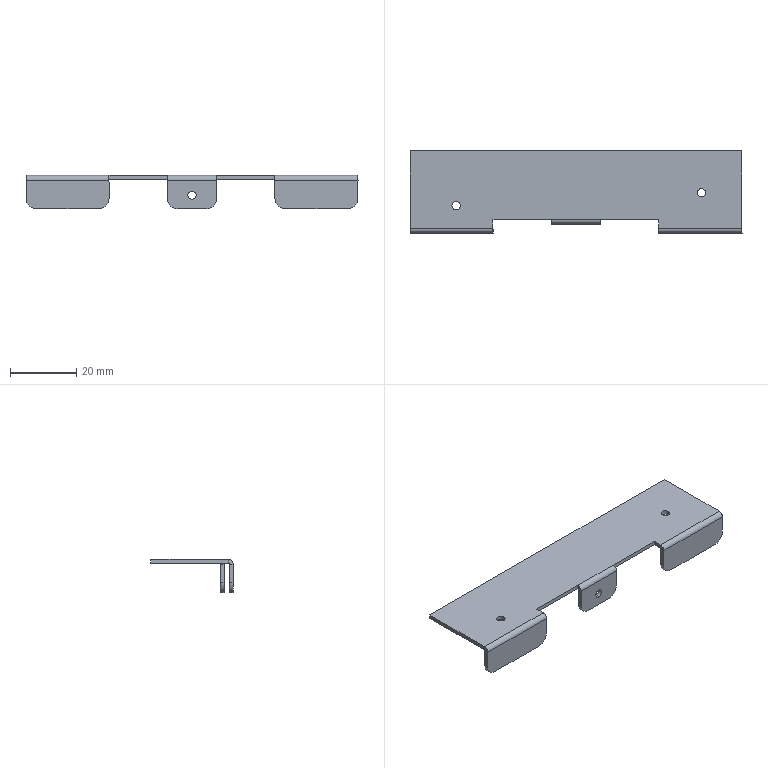Part | STEP file | 键盘盒-05^TY.NE-0002-01-014A 键盘盒-dddeger | 1 solid | 48 faces | box 100 x 24.8 x 10 mm | volume 3383 mm3 | plane 30 | cylinder 18 | commonest cylinder face diameters 2.5 x6 6 x6 0.4 x3 2.8 x3